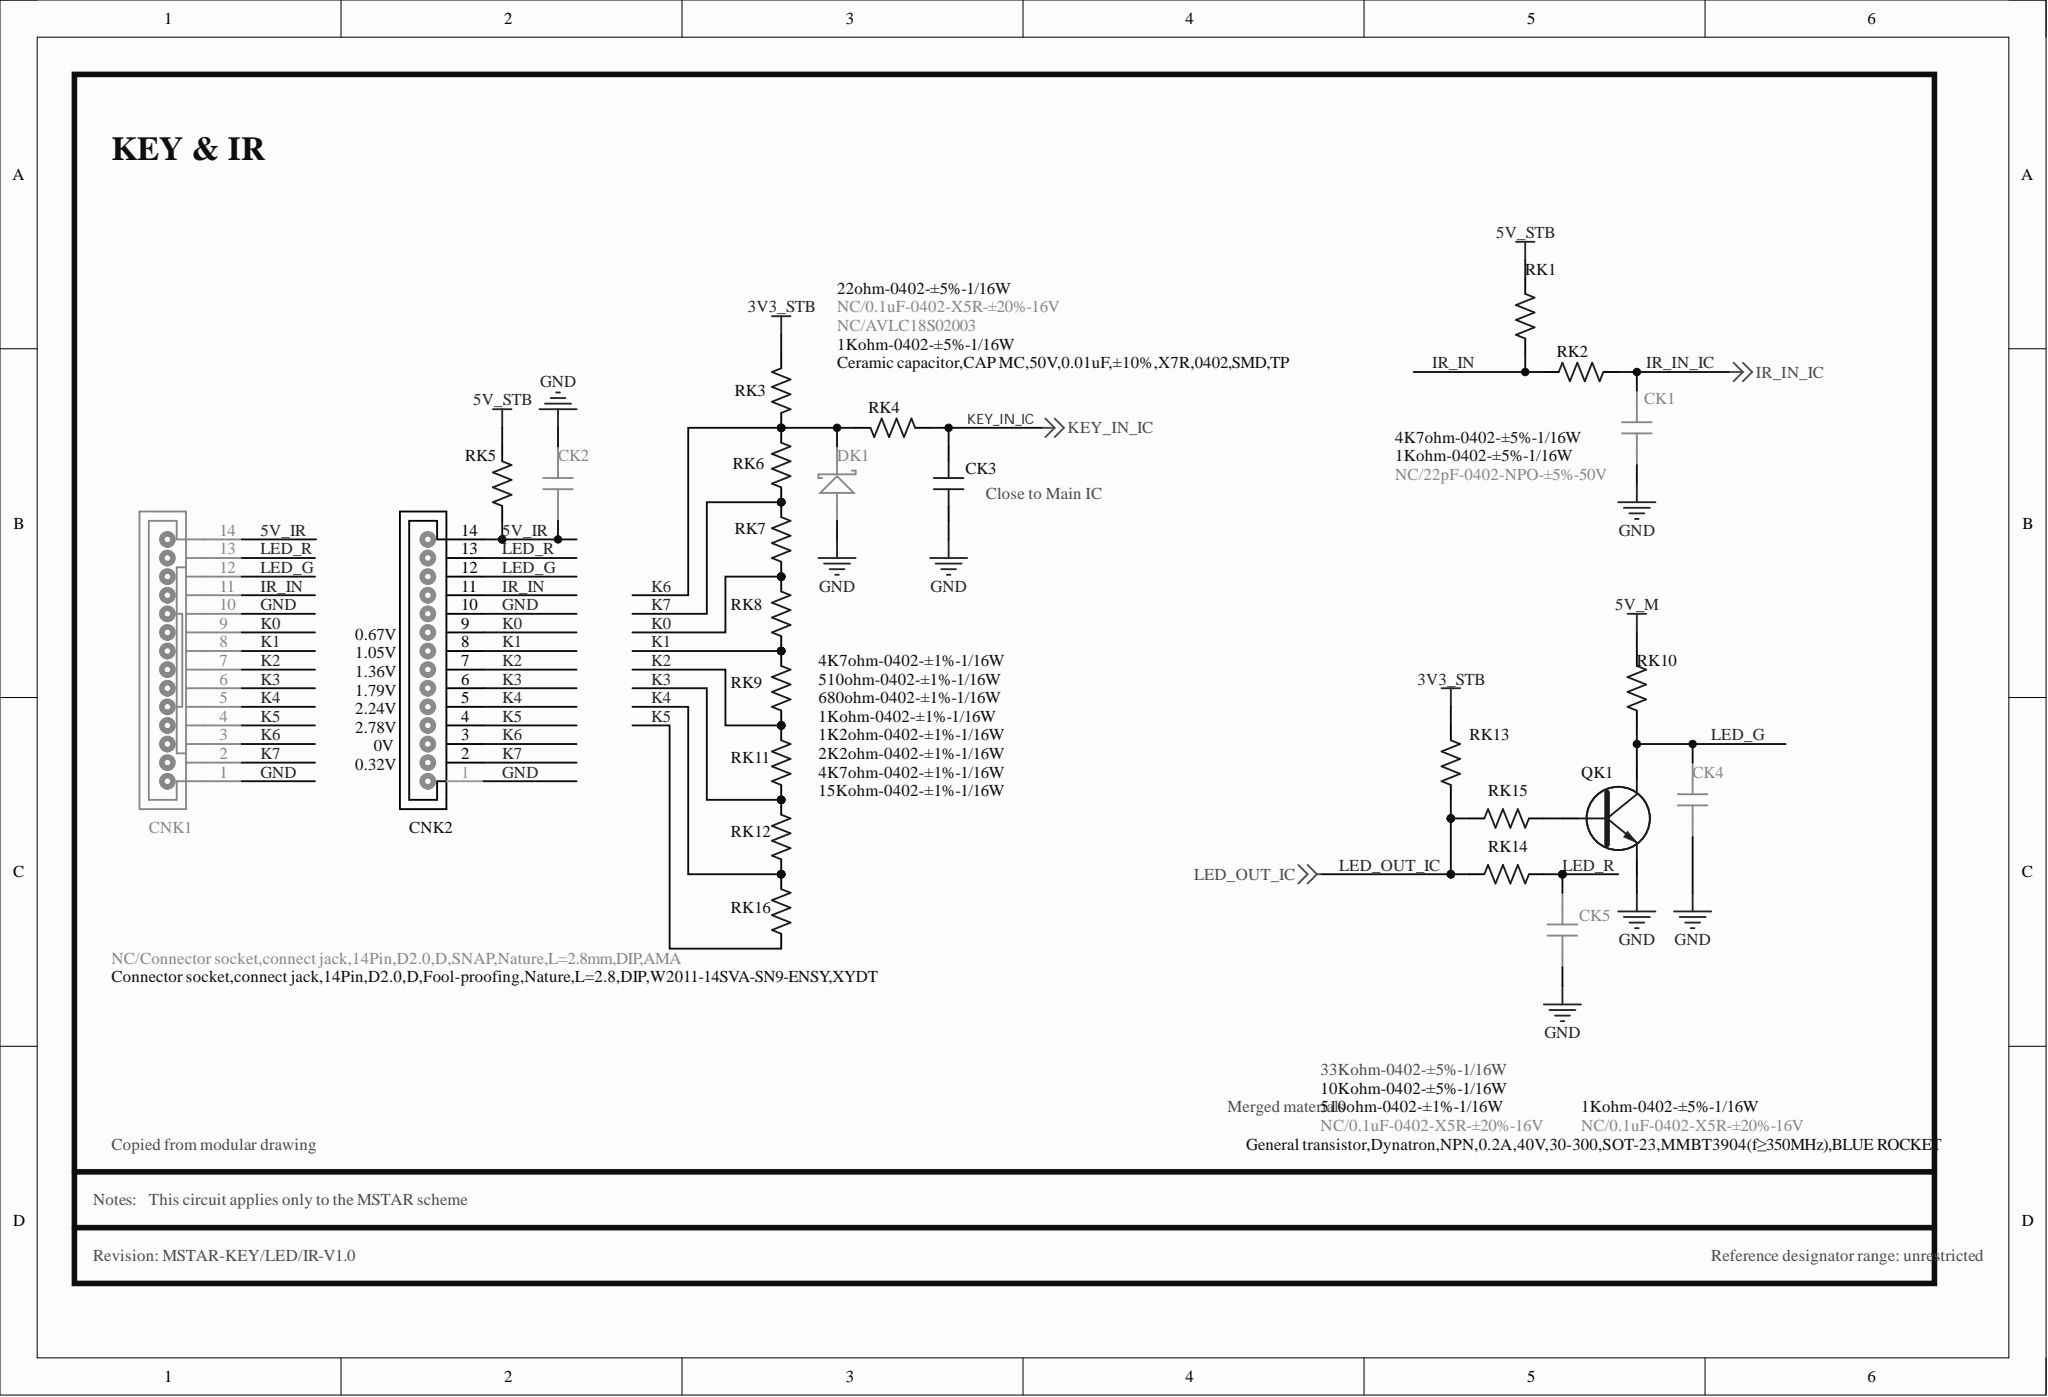Circuit board | Altium Designer | 578 parts | 300 nets | one sheet of the schematic
Parts on this sheet (reference | value | footprint):
CK1 | NC/22pF-0402-NPO-±5%-50V | C0402
CK2 | NC/0.1uF-0402-X5R-±20%-16V | C0402
CK3 | Ceramic capacitor,CAP MC,50V,0.01uF,±10%,X7R,0402,SMD,TP | C0402
CK4 | NC/0.1uF-0402-X5R-±20%-16V | C0402
CK5 | NC/0.1uF-0402-X5R-±20%-16V | C0402
CNK1 | NC/Connector socket,connect jack,14Pin,D2.0,D,SNAP,Nature,L=2.8mm,DIP,AMA | SIP14/2.0D-5
CNK2 | Connector socket,connect jack,14Pin,D2.0,D,Fool-proofing,Nature,L=2.8,DIP,W2011-14SVA-SN9-ENSY,XYDT | SIP14/2.0D-1
DK1 | NC/AVLC18S02003 | DIODE-S0402
QK1 | General transistor,Dynatron,NPN,0.2A,40V,30-300,SOT-23,MMBT3904(f=350MHz),BLUE ROCKET | SOT-23
RK1 | 4K7ohm-0402-±5%-1/16W | R0402
RK2 | 1Kohm-0402-±5%-1/16W | R0402
RK3 | 4K7ohm-0402-±1%-1/16W | R0402
RK4 | 1Kohm-0402-±5%-1/16W | R0402
RK5 | 22ohm-0402-±5%-1/16W | R0402
RK6 | 510ohm-0402-±1%-1/16W | R0402
RK7 | 680ohm-0402-±1%-1/16W | R0402
RK8 | 1Kohm-0402-±1%-1/16W | R0402
RK9 | 1K2ohm-0402-±1%-1/16W | R0402
RK10 | 1Kohm-0402-±5%-1/16W | R0402
RK11 | 2K2ohm-0402-±1%-1/16W | R0402
RK12 | 4K7ohm-0402-±1%-1/16W | R0402
RK13 | 33Kohm-0402-±5%-1/16W | R0402
RK14 | 510ohm-0402-±1%-1/16W | R0402
RK15 | 10Kohm-0402-±5%-1/16W | R0402
RK16 | 15Kohm-0402-±1%-1/16W | R0402
Nets of these parts (net: part-pin ...):
NetQK1_B: QK1-B RK15-1
LED_R: CK5-1 CNK1-13 CNK2-13 RK14-1
LED_OUT_IC: RK13-1 RK14-2 RK15-2
LED_G: CK4-1 CNK1-12 CNK2-12 QK1-C RK10-1
KEY_IN_IC: CK3-2 RK4-1
K7: CNK1-2 CNK2-2 RK6-1 RK7-2
K6: CNK1-3 CNK2-3 DK1-K RK3-1 RK4-2 RK6-2
K5: CNK1-4 CNK2-4 RK16-1
K4: CNK1-5 CNK2-5 RK12-1 RK16-2
K3: CNK1-6 CNK2-6 RK11-1 RK12-2
K2: CNK1-7 CNK2-7 RK9-1 RK11-2
K1: CNK1-8 CNK2-8 RK8-1 RK9-2
K0: CNK1-9 CNK2-9 RK7-1 RK8-2
IR_IN_IC: CK1-2 RK2-2
IR_IN: CNK1-11 CNK2-11 RK1-1 RK2-1
GND: CK1-1 CK2-1 CK3-1 CK4-2 CK5-2 CNK1-1 CNK1-10 CNK2-1 CNK2-10 DK1-A QK1-E
5V_STB: RK1-2 RK5-1
5V_M: RK10-2
5V_IR: CK2-2 CNK1-14 CNK2-14 RK5-2
3V3_STB: RK3-2 RK13-2